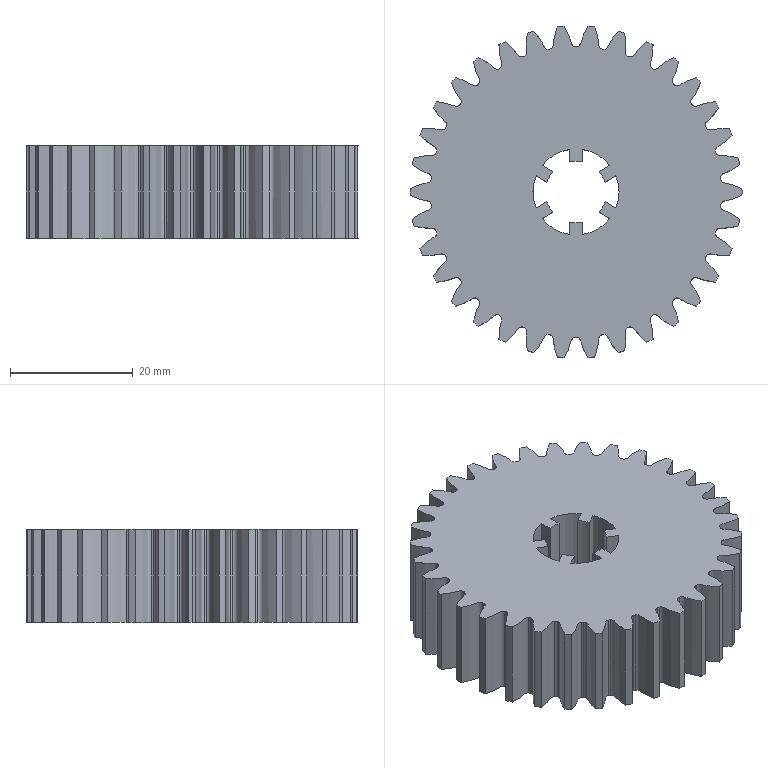Part | STEP file | 1 solid | 164 faces | box 54 x 53.862 x 15 mm | volume 28421 mm3 | cylinder 82 | spline 68 | plane 14 | commonest cylinder face diameters 54 x35 47.25 x34 14 x7 10 x6